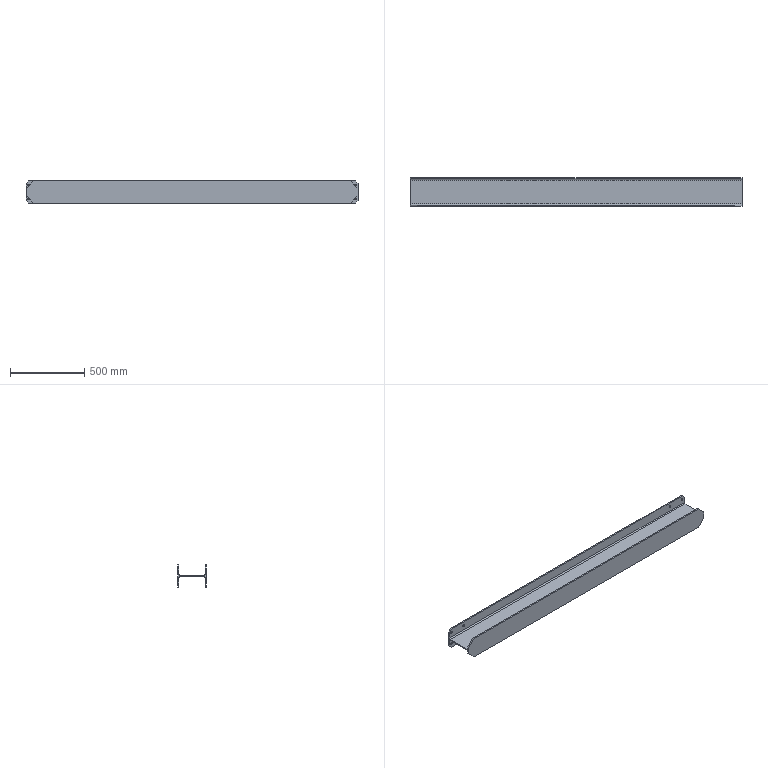Part | STEP file | E3-运输梁2-中转釜_Default<As Machined> | 1 solid | 42 faces | box 2236 x 194 x 150 mm | volume 8457974 mm3 | plane 22 | cylinder 20 | commonest cylinder face diameters 14 x16 16 x4